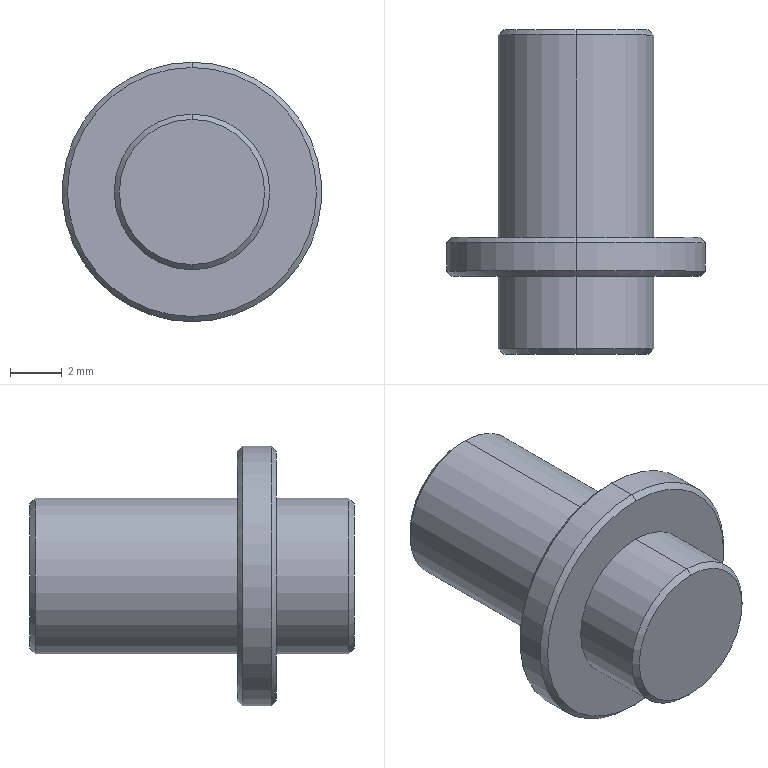Part | SolidWorks | features ICE 2, Chamfer 1, Extrusion 1 | 1 solid | 18 faces | box 10 x 12.5 x 10 mm | volume 426.85 mm3 | cone 8 | cylinder 6 | plane 4 | commonest cylinder face diameters 6 x4 10 x2
STEP:
#1=CARTESIAN_POINT('',(0.,9.5,2.8));
#2=VERTEX_POINT('',#1);
#3=CARTESIAN_POINT('',(0.,9.5,-2.8));
#4=VERTEX_POINT('',#3);
#5=CARTESIAN_POINT('',(0.,9.5,0.));
#6=DIRECTION('',(0.,1.,0.));
#7=DIRECTION('',(0.,0.,1.));
#8=AXIS2_PLACEMENT_3D('',#5,#6,#7);
#9=CIRCLE('',#8,2.8);
#10=EDGE_CURVE('',#2,#4,#9,.T.);
#11=ORIENTED_EDGE('',*,*,#10,.F.);
#12=CARTESIAN_POINT('',(0.,9.3,3.));
#13=VERTEX_POINT('',#12);
#14=CARTESIAN_POINT('',(0.,9.5,2.8));
#15=DIRECTION('',(0.,-0.7071,0.7071));
#16=VECTOR('',#15,1000.);
#17=LINE('',#14,#16);
#18=EDGE_CURVE('',#2,#13,#17,.T.);
#19=ORIENTED_EDGE('',*,*,#18,.T.);
#20=CARTESIAN_POINT('',(0.,9.3,-3.));
#21=VERTEX_POINT('',#20);
#22=CARTESIAN_POINT('',(0.,9.3,0.));
#23=DIRECTION('',(0.,-1.,0.));
#24=DIRECTION('',(0.,0.,1.));
#25=AXIS2_PLACEMENT_3D('',#22,#23,#24);
#26=CIRCLE('',#25,3.);
#27=EDGE_CURVE('',#21,#13,#26,.T.);
#28=ORIENTED_EDGE('',*,*,#27,.F.);
#29=CARTESIAN_POINT('',(0.,9.5,-2.8));
#30=DIRECTION('',(0.,-0.7071,-0.7071));
#31=VECTOR('',#30,1000.);
#32=LINE('',#29,#31);
#33=EDGE_CURVE('',#4,#21,#32,.T.);
#34=ORIENTED_EDGE('',*,*,#33,.F.);
#35=EDGE_LOOP('',(#11,#19,#28,#34));
#36=FACE_OUTER_BOUND('',#35,.T.);
#37=CARTESIAN_POINT('',(0.,9.5,0.));
#38=DIRECTION('',(0.,-1.,0.));
#39=DIRECTION('',(0.,0.,-1.));
#40=AXIS2_PLACEMENT_3D('',#37,#38,#39);
#41=CONICAL_SURFACE('',#40,2.8,0.7854);
#42=ADVANCED_FACE('',(#36),#41,.T.);
#43=CARTESIAN_POINT('',(0.,1.5,4.8));
#44=VERTEX_POINT('',#43);
#45=CARTESIAN_POINT('',(0.,1.5,-4.8));
#46=VERTEX_POINT('',#45);
#47=CARTESIAN_POINT('',(0.,1.5,0.));
#48=DIRECTION('',(0.,1.,0.));
#49=DIRECTION('',(0.,0.,1.));
#50=AXIS2_PLACEMENT_3D('',#47,#48,#49);
#51=CIRCLE('',#50,4.8);
#52=EDGE_CURVE('',#44,#46,#51,.T.);
#53=ORIENTED_EDGE('',*,*,#52,.F.);
#54=CARTESIAN_POINT('',(0.,1.3,5.));
#55=VERTEX_POINT('',#54);
#56=CARTESIAN_POINT('',(0.,1.5,4.8));
#57=DIRECTION('',(0.,-0.7071,0.7071));
#58=VECTOR('',#57,1000.);
#59=LINE('',#56,#58);
#60=EDGE_CURVE('',#44,#55,#59,.T.);
#61=ORIENTED_EDGE('',*,*,#60,.T.);
#62=CARTESIAN_POINT('',(0.,1.3,-5.));
#63=VERTEX_POINT('',#62);
#64=CARTESIAN_POINT('',(0.,1.3,0.));
#65=DIRECTION('',(0.,-1.,0.));
#66=DIRECTION('',(0.,0.,1.));
#67=AXIS2_PLACEMENT_3D('',#64,#65,#66);
#68=CIRCLE('',#67,5.);
#69=EDGE_CURVE('',#63,#55,#68,.T.);
#70=ORIENTED_EDGE('',*,*,#69,.F.);
#71=CARTESIAN_POINT('',(0.,1.5,-4.8));
#72=DIRECTION('',(0.,-0.7071,-0.7071));
#73=VECTOR('',#72,1000.);
#74=LINE('',#71,#73);
#75=EDGE_CURVE('',#46,#63,#74,.T.);
#76=ORIENTED_EDGE('',*,*,#75,.F.);
#77=EDGE_LOOP('',(#53,#61,#70,#76));
#78=FACE_OUTER_BOUND('',#77,.T.);
#79=CARTESIAN_POINT('',(0.,1.5,0.));
#80=DIRECTION('',(0.,-1.,0.));
#81=DIRECTION('',(0.,0.,-1.));
#82=AXIS2_PLACEMENT_3D('',#79,#80,#81);
#83=CONICAL_SURFACE('',#82,4.8,0.7854);
#84=ADVANCED_FACE('',(#78),#83,.T.);
#85=CARTESIAN_POINT('',(0.,0.,-4.8));
#86=VERTEX_POINT('',#85);
#87=CARTESIAN_POINT('',(0.,0.,4.8));
#88=VERTEX_POINT('',#87);
#89=CARTESIAN_POINT('',(0.,0.,0.));
#90=DIRECTION('',(0.,-1.,0.));
#91=DIRECTION('',(0.,0.,1.));
#92=AXIS2_PLACEMENT_3D('',#89,#90,#91);
#93=CIRCLE('',#92,4.8);
#94=EDGE_CURVE('',#86,#88,#93,.T.);
#95=ORIENTED_EDGE('',*,*,#94,.F.);
#96=CARTESIAN_POINT('',(0.,0.2,-5.));
#97=VERTEX_POINT('',#96);
#98=CARTESIAN_POINT('',(0.,0.2,-5.));
#99=DIRECTION('',(0.,0.7071,-0.7071));
#100=VECTOR('',#99,1000.);
#101=LINE('',#98,#100);
#102=EDGE_CURVE('',#86,#97,#101,.T.);
#103=ORIENTED_EDGE('',*,*,#102,.T.);
#104=CARTESIAN_POINT('',(0.,0.2,5.));
#105=VERTEX_POINT('',#104);
#106=CARTESIAN_POINT('',(0.,0.2,0.));
#107=DIRECTION('',(0.,1.,0.));
#108=DIRECTION('',(0.,0.,1.));
#109=AXIS2_PLACEMENT_3D('',#106,#107,#108);
#110=CIRCLE('',#109,5.);
#111=EDGE_CURVE('',#105,#97,#110,.T.);
#112=ORIENTED_EDGE('',*,*,#111,.F.);
#113=CARTESIAN_POINT('',(0.,0.2,5.));
#114=DIRECTION('',(0.,0.7071,0.7071));
#115=VECTOR('',#114,1000.);
#116=LINE('',#113,#115);
#117=EDGE_CURVE('',#88,#105,#116,.T.);
#118=ORIENTED_EDGE('',*,*,#117,.F.);
#119=EDGE_LOOP('',(#95,#103,#112,#118));
#120=FACE_OUTER_BOUND('',#119,.T.);
#121=CARTESIAN_POINT('',(0.,0.2,0.));
#122=DIRECTION('',(0.,1.,0.));
#123=DIRECTION('',(0.,0.,1.));
#124=AXIS2_PLACEMENT_3D('',#121,#122,#123);
#125=CONICAL_SURFACE('',#124,5.,0.7854);
#126=ADVANCED_FACE('',(#120),#125,.T.);
#127=CARTESIAN_POINT('',(0.,-3.,-2.8));
#128=VERTEX_POINT('',#127);
#129=CARTESIAN_POINT('',(0.,-3.,2.8));
#130=VERTEX_POINT('',#129);
#131=CARTESIAN_POINT('',(0.,-3.,0.));
#132=DIRECTION('',(0.,-1.,0.));
#133=DIRECTION('',(0.,0.,-1.));
#134=AXIS2_PLACEMENT_3D('',#131,#132,#133);
#135=CIRCLE('',#134,2.8);
#136=EDGE_CURVE('',#128,#130,#135,.T.);
#137=ORIENTED_EDGE('',*,*,#136,.F.);
#138=CARTESIAN_POINT('',(0.,-2.8,-3.));
#139=VERTEX_POINT('',#138);
#140=CARTESIAN_POINT('',(0.,-3.,-2.8));
#141=DIRECTION('',(0.,0.7071,-0.7071));
#142=VECTOR('',#141,1000.);
#143=LINE('',#140,#142);
#144=EDGE_CURVE('',#128,#139,#143,.T.);
#145=ORIENTED_EDGE('',*,*,#144,.T.);
#146=CARTESIAN_POINT('',(0.,-2.8,3.));
#147=VERTEX_POINT('',#146);
#148=CARTESIAN_POINT('',(0.,-2.8,0.));
#149=DIRECTION('',(0.,1.,0.));
#150=DIRECTION('',(0.,0.,-1.));
#151=AXIS2_PLACEMENT_3D('',#148,#149,#150);
#152=CIRCLE('',#151,3.);
#153=EDGE_CURVE('',#147,#139,#152,.T.);
#154=ORIENTED_EDGE('',*,*,#153,.F.);
#155=CARTESIAN_POINT('',(0.,-3.,2.8));
#156=DIRECTION('',(0.,0.7071,0.7071));
#157=VECTOR('',#156,1000.);
#158=LINE('',#155,#157);
#159=EDGE_CURVE('',#130,#147,#158,.T.);
#160=ORIENTED_EDGE('',*,*,#159,.F.);
#161=EDGE_LOOP('',(#137,#145,#154,#160));
#162=FACE_OUTER_BOUND('',#161,.T.);
#163=CARTESIAN_POINT('',(0.,-3.,0.));
#164=DIRECTION('',(0.,1.,0.));
#165=DIRECTION('',(0.,0.,1.));
#166=AXIS2_PLACEMENT_3D('',#163,#164,#165);
#167=CONICAL_SURFACE('',#166,2.8,0.7854);
#168=ADVANCED_FACE('',(#162),#167,.T.);
#169=ORIENTED_EDGE('',*,*,#153,.T.);
#170=CARTESIAN_POINT('',(0.,0.,-3.));
#171=VERTEX_POINT('',#170);
#172=CARTESIAN_POINT('',(0.,-3.,-3.));
#173=DIRECTION('',(0.,1.,0.));
#174=VECTOR('',#173,1000.);
#175=LINE('',#172,#174);
#176=EDGE_CURVE('',#139,#171,#175,.T.);
#177=ORIENTED_EDGE('',*,*,#176,.T.);
#178=CARTESIAN_POINT('',(0.,0.,3.));
#179=VERTEX_POINT('',#178);
#180=CARTESIAN_POINT('',(0.,0.,0.));
#181=DIRECTION('',(0.,-1.,0.));
#182=DIRECTION('',(0.,0.,1.));
#183=AXIS2_PLACEMENT_3D('',#180,#181,#182);
#184=CIRCLE('',#183,3.);
#185=EDGE_CURVE('',#171,#179,#184,.T.);
#186=ORIENTED_EDGE('',*,*,#185,.T.);
#187=CARTESIAN_POINT('',(0.,-3.,3.));
#188=DIRECTION('',(0.,1.,0.));
#189=VECTOR('',#188,1000.);
#190=LINE('',#187,#189);
#191=EDGE_CURVE('',#147,#179,#190,.T.);
#192=ORIENTED_EDGE('',*,*,#191,.F.);
#193=EDGE_LOOP('',(#169,#177,#186,#192));
#194=FACE_OUTER_BOUND('',#193,.T.);
#195=CARTESIAN_POINT('',(0.,-3.,0.));
#196=DIRECTION('',(0.,1.,0.));
#197=DIRECTION('',(0.,0.,1.));
#198=AXIS2_PLACEMENT_3D('',#195,#196,#197);
#199=CYLINDRICAL_SURFACE('',#198,3.);
#200=ADVANCED_FACE('',(#194),#199,.T.);
#201=ORIENTED_EDGE('',*,*,#27,.T.);
#202=CARTESIAN_POINT('',(0.,1.5,3.));
#203=VERTEX_POINT('',#202);
#204=CARTESIAN_POINT('',(0.,9.5,3.));
#205=DIRECTION('',(0.,-1.,0.));
#206=VECTOR('',#205,1000.);
#207=LINE('',#204,#206);
#208=EDGE_CURVE('',#13,#203,#207,.T.);
#209=ORIENTED_EDGE('',*,*,#208,.T.);
#210=CARTESIAN_POINT('',(0.,1.5,-3.));
#211=VERTEX_POINT('',#210);
#212=CARTESIAN_POINT('',(0.,1.5,0.));
#213=DIRECTION('',(0.,1.,0.));
#214=DIRECTION('',(0.,0.,1.));
#215=AXIS2_PLACEMENT_3D('',#212,#213,#214);
#216=CIRCLE('',#215,3.);
#217=EDGE_CURVE('',#203,#211,#216,.T.);
#218=ORIENTED_EDGE('',*,*,#217,.T.);
#219=CARTESIAN_POINT('',(0.,9.5,-3.));
#220=DIRECTION('',(0.,-1.,0.));
#221=VECTOR('',#220,1000.);
#222=LINE('',#219,#221);
#223=EDGE_CURVE('',#21,#211,#222,.T.);
#224=ORIENTED_EDGE('',*,*,#223,.F.);
#225=EDGE_LOOP('',(#201,#209,#218,#224));
#226=FACE_OUTER_BOUND('',#225,.T.);
#227=CARTESIAN_POINT('',(0.,9.5,0.));
#228=DIRECTION('',(0.,-1.,0.));
#229=DIRECTION('',(0.,0.,-1.));
#230=AXIS2_PLACEMENT_3D('',#227,#228,#229);
#231=CYLINDRICAL_SURFACE('',#230,3.);
#232=ADVANCED_FACE('',(#226),#231,.T.);
#233=ORIENTED_EDGE('',*,*,#69,.T.);
#234=CARTESIAN_POINT('',(0.,1.5,5.));
#235=DIRECTION('',(0.,-1.,0.));
#236=VECTOR('',#235,1000.);
#237=LINE('',#234,#236);
#238=EDGE_CURVE('',#55,#105,#237,.T.);
#239=ORIENTED_EDGE('',*,*,#238,.T.);
#240=ORIENTED_EDGE('',*,*,#111,.T.);
#241=CARTESIAN_POINT('',(0.,1.5,-5.));
#242=DIRECTION('',(0.,-1.,0.));
#243=VECTOR('',#242,1000.);
#244=LINE('',#241,#243);
#245=EDGE_CURVE('',#63,#97,#244,.T.);
#246=ORIENTED_EDGE('',*,*,#245,.F.);
#247=EDGE_LOOP('',(#233,#239,#240,#246));
#248=FACE_OUTER_BOUND('',#247,.T.);
#249=CARTESIAN_POINT('',(0.,1.5,0.));
#250=DIRECTION('',(0.,-1.,0.));
#251=DIRECTION('',(0.,0.,-1.));
#252=AXIS2_PLACEMENT_3D('',#249,#250,#251);
#253=CYLINDRICAL_SURFACE('',#252,5.);
#254=ADVANCED_FACE('',(#248),#253,.T.);
#255=CARTESIAN_POINT('',(0.,0.,0.));
#256=DIRECTION('',(0.,-1.,0.));
#257=DIRECTION('',(0.,0.,1.));
#258=AXIS2_PLACEMENT_3D('',#255,#256,#257);
#259=CIRCLE('',#258,4.8);
#260=EDGE_CURVE('',#88,#86,#259,.T.);
#261=ORIENTED_EDGE('',*,*,#260,.T.);
#262=ORIENTED_EDGE('',*,*,#94,.T.);
#263=EDGE_LOOP('',(#261,#262));
#264=FACE_OUTER_BOUND('',#263,.T.);
#265=CARTESIAN_POINT('',(0.,0.,0.));
#266=DIRECTION('',(0.,-1.,0.));
#267=DIRECTION('',(0.,0.,1.));
#268=AXIS2_PLACEMENT_3D('',#265,#266,#267);
#269=CIRCLE('',#268,3.);
#270=EDGE_CURVE('',#179,#171,#269,.T.);
#271=ORIENTED_EDGE('',*,*,#270,.F.);
#272=ORIENTED_EDGE('',*,*,#185,.F.);
#273=EDGE_LOOP('',(#271,#272));
#274=FACE_BOUND('',#273,.T.);
#275=CARTESIAN_POINT('',(0.,0.,0.));
#276=DIRECTION('',(0.,1.,0.));
#277=DIRECTION('',(0.,0.,1.));
#278=AXIS2_PLACEMENT_3D('',#275,#276,#277);
#279=PLANE('',#278);
#280=ADVANCED_FACE('',(#264,#274),#279,.F.);
#281=CARTESIAN_POINT('',(0.,1.5,0.));
#282=DIRECTION('',(0.,1.,0.));
#283=DIRECTION('',(0.,0.,1.));
#284=AXIS2_PLACEMENT_3D('',#281,#282,#283);
#285=CIRCLE('',#284,4.8);
#286=EDGE_CURVE('',#46,#44,#285,.T.);
#287=ORIENTED_EDGE('',*,*,#286,.T.);
#288=ORIENTED_EDGE('',*,*,#52,.T.);
#289=EDGE_LOOP('',(#287,#288));
#290=FACE_OUTER_BOUND('',#289,.T.);
#291=CARTESIAN_POINT('',(0.,1.5,0.));
#292=DIRECTION('',(0.,1.,0.));
#293=DIRECTION('',(0.,0.,1.));
#294=AXIS2_PLACEMENT_3D('',#291,#292,#293);
#295=CIRCLE('',#294,3.);
#296=EDGE_CURVE('',#211,#203,#295,.T.);
#297=ORIENTED_EDGE('',*,*,#296,.F.);
#298=ORIENTED_EDGE('',*,*,#217,.F.);
#299=EDGE_LOOP('',(#297,#298));
#300=FACE_BOUND('',#299,.T.);
#301=CARTESIAN_POINT('',(0.,1.5,0.));
#302=DIRECTION('',(0.,1.,0.));
#303=DIRECTION('',(0.,0.,1.));
#304=AXIS2_PLACEMENT_3D('',#301,#302,#303);
#305=PLANE('',#304);
#306=ADVANCED_FACE('',(#290,#300),#305,.T.);
#307=ORIENTED_EDGE('',*,*,#238,.F.);
#308=CARTESIAN_POINT('',(0.,1.3,0.));
#309=DIRECTION('',(0.,-1.,0.));
#310=DIRECTION('',(0.,0.,1.));
#311=AXIS2_PLACEMENT_3D('',#308,#309,#310);
#312=CIRCLE('',#311,5.);
#313=EDGE_CURVE('',#55,#63,#312,.T.);
#314=ORIENTED_EDGE('',*,*,#313,.T.);
#315=ORIENTED_EDGE('',*,*,#245,.T.);
#316=CARTESIAN_POINT('',(0.,0.2,0.));
#317=DIRECTION('',(0.,1.,0.));
#318=DIRECTION('',(0.,0.,1.));
#319=AXIS2_PLACEMENT_3D('',#316,#317,#318);
#320=CIRCLE('',#319,5.);
#321=EDGE_CURVE('',#97,#105,#320,.T.);
#322=ORIENTED_EDGE('',*,*,#321,.T.);
#323=EDGE_LOOP('',(#307,#314,#315,#322));
#324=FACE_OUTER_BOUND('',#323,.T.);
#325=CARTESIAN_POINT('',(0.,1.5,0.));
#326=DIRECTION('',(0.,-1.,0.));
#327=DIRECTION('',(0.,0.,-1.));
#328=AXIS2_PLACEMENT_3D('',#325,#326,#327);
#329=CYLINDRICAL_SURFACE('',#328,5.);
#330=ADVANCED_FACE('',(#324),#329,.T.);
#331=ORIENTED_EDGE('',*,*,#208,.F.);
#332=CARTESIAN_POINT('',(0.,9.3,0.));
#333=DIRECTION('',(0.,-1.,0.));
#334=DIRECTION('',(0.,0.,1.));
#335=AXIS2_PLACEMENT_3D('',#332,#333,#334);
#336=CIRCLE('',#335,3.);
#337=EDGE_CURVE('',#13,#21,#336,.T.);
#338=ORIENTED_EDGE('',*,*,#337,.T.);
#339=ORIENTED_EDGE('',*,*,#223,.T.);
#340=ORIENTED_EDGE('',*,*,#296,.T.);
#341=EDGE_LOOP('',(#331,#338,#339,#340));
#342=FACE_OUTER_BOUND('',#341,.T.);
#343=CARTESIAN_POINT('',(0.,9.5,0.));
#344=DIRECTION('',(0.,-1.,0.));
#345=DIRECTION('',(0.,0.,-1.));
#346=AXIS2_PLACEMENT_3D('',#343,#344,#345);
#347=CYLINDRICAL_SURFACE('',#346,3.);
#348=ADVANCED_FACE('',(#342),#347,.T.);
#349=CARTESIAN_POINT('',(0.,9.5,0.));
#350=DIRECTION('',(0.,1.,0.));
#351=DIRECTION('',(0.,0.,1.));
#352=AXIS2_PLACEMENT_3D('',#349,#350,#351);
#353=CIRCLE('',#352,2.8);
#354=EDGE_CURVE('',#4,#2,#353,.T.);
#355=ORIENTED_EDGE('',*,*,#354,.T.);
#356=ORIENTED_EDGE('',*,*,#10,.T.);
#357=EDGE_LOOP('',(#355,#356));
#358=FACE_OUTER_BOUND('',#357,.T.);
#359=CARTESIAN_POINT('',(0.,9.5,0.));
#360=DIRECTION('',(0.,1.,0.));
#361=DIRECTION('',(0.,0.,1.));
#362=AXIS2_PLACEMENT_3D('',#359,#360,#361);
#363=PLANE('',#362);
#364=ADVANCED_FACE('',(#358),#363,.T.);
#365=ORIENTED_EDGE('',*,*,#176,.F.);
#366=CARTESIAN_POINT('',(0.,-2.8,0.));
#367=DIRECTION('',(0.,1.,0.));
#368=DIRECTION('',(0.,0.,-1.));
#369=AXIS2_PLACEMENT_3D('',#366,#367,#368);
#370=CIRCLE('',#369,3.);
#371=EDGE_CURVE('',#139,#147,#370,.T.);
#372=ORIENTED_EDGE('',*,*,#371,.T.);
#373=ORIENTED_EDGE('',*,*,#191,.T.);
#374=ORIENTED_EDGE('',*,*,#270,.T.);
#375=EDGE_LOOP('',(#365,#372,#373,#374));
#376=FACE_OUTER_BOUND('',#375,.T.);
#377=CARTESIAN_POINT('',(0.,-3.,0.));
#378=DIRECTION('',(0.,1.,0.));
#379=DIRECTION('',(0.,0.,1.));
#380=AXIS2_PLACEMENT_3D('',#377,#378,#379);
#381=CYLINDRICAL_SURFACE('',#380,3.);
#382=ADVANCED_FACE('',(#376),#381,.T.);
#383=CARTESIAN_POINT('',(0.,-3.,0.));
#384=DIRECTION('',(0.,-1.,0.));
#385=DIRECTION('',(0.,0.,-1.));
#386=AXIS2_PLACEMENT_3D('',#383,#384,#385);
#387=CIRCLE('',#386,2.8);
#388=EDGE_CURVE('',#130,#128,#387,.T.);
#389=ORIENTED_EDGE('',*,*,#388,.T.);
#390=ORIENTED_EDGE('',*,*,#136,.T.);
#391=EDGE_LOOP('',(#389,#390));
#392=FACE_OUTER_BOUND('',#391,.T.);
#393=CARTESIAN_POINT('',(0.,-3.,0.));
#394=DIRECTION('',(0.,-1.,0.));
#395=DIRECTION('',(0.,0.,-1.));
#396=AXIS2_PLACEMENT_3D('',#393,#394,#395);
#397=PLANE('',#396);
#398=ADVANCED_FACE('',(#392),#397,.T.);
#399=ORIENTED_EDGE('',*,*,#144,.F.);
#400=ORIENTED_EDGE('',*,*,#388,.F.);
#401=ORIENTED_EDGE('',*,*,#159,.T.);
#402=ORIENTED_EDGE('',*,*,#371,.F.);
#403=EDGE_LOOP('',(#399,#400,#401,#402));
#404=FACE_OUTER_BOUND('',#403,.T.);
#405=CARTESIAN_POINT('',(0.,-3.,0.));
#406=DIRECTION('',(0.,1.,0.));
#407=DIRECTION('',(0.,0.,1.));
#408=AXIS2_PLACEMENT_3D('',#405,#406,#407);
#409=CONICAL_SURFACE('',#408,2.8,0.7854);
#410=ADVANCED_FACE('',(#404),#409,.T.);
#411=ORIENTED_EDGE('',*,*,#102,.F.);
#412=ORIENTED_EDGE('',*,*,#260,.F.);
#413=ORIENTED_EDGE('',*,*,#117,.T.);
#414=ORIENTED_EDGE('',*,*,#321,.F.);
#415=EDGE_LOOP('',(#411,#412,#413,#414));
#416=FACE_OUTER_BOUND('',#415,.T.);
#417=CARTESIAN_POINT('',(0.,0.2,0.));
#418=DIRECTION('',(0.,1.,0.));
#419=DIRECTION('',(0.,0.,1.));
#420=AXIS2_PLACEMENT_3D('',#417,#418,#419);
#421=CONICAL_SURFACE('',#420,5.,0.7854);
#422=ADVANCED_FACE('',(#416),#421,.T.);
#423=ORIENTED_EDGE('',*,*,#60,.F.);
#424=ORIENTED_EDGE('',*,*,#286,.F.);
#425=ORIENTED_EDGE('',*,*,#75,.T.);
#426=ORIENTED_EDGE('',*,*,#313,.F.);
#427=EDGE_LOOP('',(#423,#424,#425,#426));
#428=FACE_OUTER_BOUND('',#427,.T.);
#429=CARTESIAN_POINT('',(0.,1.5,0.));
#430=DIRECTION('',(0.,-1.,0.));
#431=DIRECTION('',(0.,0.,-1.));
#432=AXIS2_PLACEMENT_3D('',#429,#430,#431);
#433=CONICAL_SURFACE('',#432,4.8,0.7854);
#434=ADVANCED_FACE('',(#428),#433,.T.);
#435=ORIENTED_EDGE('',*,*,#18,.F.);
#436=ORIENTED_EDGE('',*,*,#354,.F.);
#437=ORIENTED_EDGE('',*,*,#33,.T.);
#438=ORIENTED_EDGE('',*,*,#337,.F.);
#439=EDGE_LOOP('',(#435,#436,#437,#438));
#440=FACE_OUTER_BOUND('',#439,.T.);
#441=CARTESIAN_POINT('',(0.,9.5,0.));
#442=DIRECTION('',(0.,-1.,0.));
#443=DIRECTION('',(0.,0.,-1.));
#444=AXIS2_PLACEMENT_3D('',#441,#442,#443);
#445=CONICAL_SURFACE('',#444,2.8,0.7854);
#446=ADVANCED_FACE('',(#440),#445,.T.);
#447=CLOSED_SHELL('',(#42,#84,#126,#168,#200,#232,#254,#280,#306,#330,#348,#364,#382,#398,#410,#422,#434,#446));
#448=MANIFOLD_SOLID_BREP('',#447);
#449=CARTESIAN_POINT('',(0.,0.,0.));
#450=DIRECTION('',(0.,0.,1.));
#451=DIRECTION('',(1.,0.,0.));
#452=AXIS2_PLACEMENT_3D('',#449,#450,#451);
#453=(LENGTH_UNIT()NAMED_UNIT(*)SI_UNIT(.MILLI.,.METRE.));
#454=UNCERTAINTY_MEASURE_WITH_UNIT(LENGTH_MEASURE(0.00001),#453,'','');
#455=(NAMED_UNIT(*)PLANE_ANGLE_UNIT()SI_UNIT($,.RADIAN.));
#456=(NAMED_UNIT(*)SI_UNIT($,.STERADIAN.)SOLID_ANGLE_UNIT());
#457=(GEOMETRIC_REPRESENTATION_CONTEXT(3)GLOBAL_UNCERTAINTY_ASSIGNED_CONTEXT((#454))GLOBAL_UNIT_ASSIGNED_CONTEXT((#453,#455,#456))REPRESENTATION_CONTEXT('',''));
#458=ADVANCED_BREP_SHAPE_REPRESENTATION('',(#448,#452),#457);